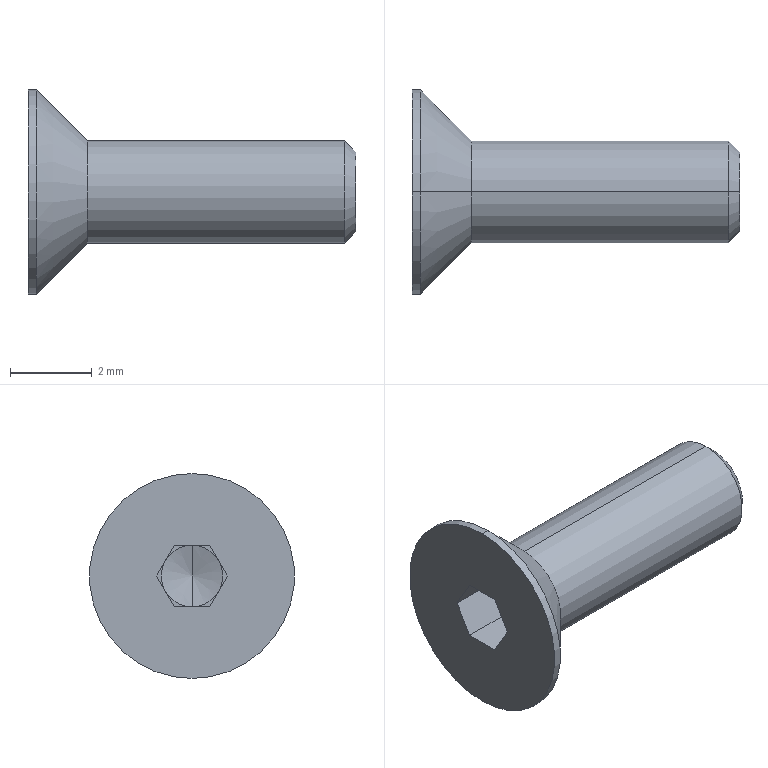Part | STEP file | 11-FG99-FBa2_5_8-V3.0-kkkkkk-998.11 | 1 solid | 24 faces | box 8 x 5 x 5 mm | volume 47.741 mm3 | plane 14 | cone 6 | cylinder 4 | commonest cylinder face diameters 2.5 x2 5 x2
STEP:
#1=CARTESIAN_POINT('',(1.361,0.,0.));
#2=VERTEX_POINT('',#1);
#3=CARTESIAN_POINT('',(1.16,0.,0.75));
#4=VERTEX_POINT('',#3);
#5=CARTESIAN_POINT('',(1.361,0.,0.));
#6=DIRECTION('',(-0.2588,0.,0.9659));
#7=VECTOR('',#6,1000.);
#8=LINE('',#5,#7);
#9=EDGE_CURVE('',#2,#4,#8,.T.);
#10=ORIENTED_EDGE('',*,*,#9,.F.);
#11=CARTESIAN_POINT('',(1.16,0.,-0.75));
#12=VERTEX_POINT('',#11);
#13=CARTESIAN_POINT('',(1.361,0.,0.));
#14=DIRECTION('',(-0.2588,0.,-0.9659));
#15=VECTOR('',#14,1000.);
#16=LINE('',#13,#15);
#17=EDGE_CURVE('',#2,#12,#16,.T.);
#18=ORIENTED_EDGE('',*,*,#17,.T.);
#19=CARTESIAN_POINT('',(1.16,-0.6495,-0.375));
#20=VERTEX_POINT('',#19);
#21=CARTESIAN_POINT('',(1.16,0.,0.));
#22=DIRECTION('',(-1.,0.,0.));
#23=DIRECTION('',(0.,0.,1.));
#24=AXIS2_PLACEMENT_3D('',#21,#22,#23);
#25=CIRCLE('',#24,0.75);
#26=EDGE_CURVE('',#12,#20,#25,.T.);
#27=ORIENTED_EDGE('',*,*,#26,.T.);
#28=CARTESIAN_POINT('',(1.16,-0.6495,0.375));
#29=VERTEX_POINT('',#28);
#30=CARTESIAN_POINT('',(1.16,0.,0.));
#31=DIRECTION('',(-1.,0.,0.));
#32=DIRECTION('',(0.,0.,1.));
#33=AXIS2_PLACEMENT_3D('',#30,#31,#32);
#34=CIRCLE('',#33,0.75);
#35=EDGE_CURVE('',#20,#29,#34,.T.);
#36=ORIENTED_EDGE('',*,*,#35,.T.);
#37=CARTESIAN_POINT('',(1.16,0.,0.));
#38=DIRECTION('',(-1.,0.,0.));
#39=DIRECTION('',(0.,0.,1.));
#40=AXIS2_PLACEMENT_3D('',#37,#38,#39);
#41=CIRCLE('',#40,0.75);
#42=EDGE_CURVE('',#29,#4,#41,.T.);
#43=ORIENTED_EDGE('',*,*,#42,.T.);
#44=EDGE_LOOP('',(#10,#18,#27,#36,#43));
#45=FACE_OUTER_BOUND('',#44,.T.);
#46=CARTESIAN_POINT('',(-998.639,0.,0.));
#47=DIRECTION('',(-1.,0.,0.));
#48=DIRECTION('',(0.,0.,1.));
#49=AXIS2_PLACEMENT_3D('',#46,#47,#48);
#50=CONICAL_SURFACE('',#49,3732.051,1.309);
#51=ADVANCED_FACE('',(#45),#50,.F.);
#52=CARTESIAN_POINT('',(8.,0.,0.974));
#53=VERTEX_POINT('',#52);
#54=CARTESIAN_POINT('',(8.,0.,-0.974));
#55=VERTEX_POINT('',#54);
#56=CARTESIAN_POINT('',(8.,0.,0.));
#57=DIRECTION('',(-1.,0.,0.));
#58=DIRECTION('',(0.,0.,1.));
#59=AXIS2_PLACEMENT_3D('',#56,#57,#58);
#60=CIRCLE('',#59,0.974);
#61=EDGE_CURVE('',#53,#55,#60,.T.);
#62=ORIENTED_EDGE('',*,*,#61,.T.);
#63=CARTESIAN_POINT('',(7.724,0.,-1.25));
#64=VERTEX_POINT('',#63);
#65=CARTESIAN_POINT('',(8.,0.,-0.974));
#66=DIRECTION('',(-0.7071,0.,-0.7071));
#67=VECTOR('',#66,1000.);
#68=LINE('',#65,#67);
#69=EDGE_CURVE('',#55,#64,#68,.T.);
#70=ORIENTED_EDGE('',*,*,#69,.T.);
#71=CARTESIAN_POINT('',(7.724,0.,1.25));
#72=VERTEX_POINT('',#71);
#73=CARTESIAN_POINT('',(7.724,0.,0.));
#74=DIRECTION('',(-1.,0.,0.));
#75=DIRECTION('',(0.,0.,1.));
#76=AXIS2_PLACEMENT_3D('',#73,#74,#75);
#77=CIRCLE('',#76,1.25);
#78=EDGE_CURVE('',#72,#64,#77,.T.);
#79=ORIENTED_EDGE('',*,*,#78,.F.);
#80=CARTESIAN_POINT('',(8.,0.,0.974));
#81=DIRECTION('',(-0.7071,0.,0.7071));
#82=VECTOR('',#81,1000.);
#83=LINE('',#80,#82);
#84=EDGE_CURVE('',#53,#72,#83,.T.);
#85=ORIENTED_EDGE('',*,*,#84,.F.);
#86=EDGE_LOOP('',(#62,#70,#79,#85));
#87=FACE_OUTER_BOUND('',#86,.T.);
#88=CARTESIAN_POINT('',(8.,0.,0.));
#89=DIRECTION('',(-1.,0.,0.));
#90=DIRECTION('',(0.,0.,1.));
#91=AXIS2_PLACEMENT_3D('',#88,#89,#90);
#92=CONICAL_SURFACE('',#91,0.974,0.7854);
#93=ADVANCED_FACE('',(#87),#92,.T.);
#94=ORIENTED_EDGE('',*,*,#78,.T.);
#95=CARTESIAN_POINT('',(1.45,0.,-1.25));
#96=VERTEX_POINT('',#95);
#97=CARTESIAN_POINT('',(8.,0.,-1.25));
#98=DIRECTION('',(-1.,0.,0.));
#99=VECTOR('',#98,1000.);
#100=LINE('',#97,#99);
#101=EDGE_CURVE('',#64,#96,#100,.T.);
#102=ORIENTED_EDGE('',*,*,#101,.T.);
#103=CARTESIAN_POINT('',(1.45,0.,1.25));
#104=VERTEX_POINT('',#103);
#105=CARTESIAN_POINT('',(1.45,0.,0.));
#106=DIRECTION('',(-1.,0.,0.));
#107=DIRECTION('',(0.,0.,1.));
#108=AXIS2_PLACEMENT_3D('',#105,#106,#107);
#109=CIRCLE('',#108,1.25);
#110=EDGE_CURVE('',#104,#96,#109,.T.);
#111=ORIENTED_EDGE('',*,*,#110,.F.);
#112=CARTESIAN_POINT('',(8.,0.,1.25));
#113=DIRECTION('',(-1.,0.,0.));
#114=VECTOR('',#113,1000.);
#115=LINE('',#112,#114);
#116=EDGE_CURVE('',#72,#104,#115,.T.);
#117=ORIENTED_EDGE('',*,*,#116,.F.);
#118=EDGE_LOOP('',(#94,#102,#111,#117));
#119=FACE_OUTER_BOUND('',#118,.T.);
#120=CARTESIAN_POINT('',(8.,0.,0.));
#121=DIRECTION('',(-1.,0.,0.));
#122=DIRECTION('',(0.,0.,1.));
#123=AXIS2_PLACEMENT_3D('',#120,#121,#122);
#124=CYLINDRICAL_SURFACE('',#123,1.25);
#125=ADVANCED_FACE('',(#119),#124,.T.);
#126=ORIENTED_EDGE('',*,*,#110,.T.);
#127=CARTESIAN_POINT('',(0.2,0.,-2.5));
#128=VERTEX_POINT('',#127);
#129=CARTESIAN_POINT('',(1.45,0.,-1.25));
#130=DIRECTION('',(-0.7071,0.,-0.7071));
#131=VECTOR('',#130,1000.);
#132=LINE('',#129,#131);
#133=EDGE_CURVE('',#96,#128,#132,.T.);
#134=ORIENTED_EDGE('',*,*,#133,.T.);
#135=CARTESIAN_POINT('',(0.2,0.,2.5));
#136=VERTEX_POINT('',#135);
#137=CARTESIAN_POINT('',(0.2,0.,0.));
#138=DIRECTION('',(-1.,0.,0.));
#139=DIRECTION('',(0.,0.,1.));
#140=AXIS2_PLACEMENT_3D('',#137,#138,#139);
#141=CIRCLE('',#140,2.5);
#142=EDGE_CURVE('',#136,#128,#141,.T.);
#143=ORIENTED_EDGE('',*,*,#142,.F.);
#144=CARTESIAN_POINT('',(1.45,0.,1.25));
#145=DIRECTION('',(-0.7071,0.,0.7071));
#146=VECTOR('',#145,1000.);
#147=LINE('',#144,#146);
#148=EDGE_CURVE('',#104,#136,#147,.T.);
#149=ORIENTED_EDGE('',*,*,#148,.F.);
#150=EDGE_LOOP('',(#126,#134,#143,#149));
#151=FACE_OUTER_BOUND('',#150,.T.);
#152=CARTESIAN_POINT('',(1.45,0.,0.));
#153=DIRECTION('',(-1.,0.,0.));
#154=DIRECTION('',(0.,0.,1.));
#155=AXIS2_PLACEMENT_3D('',#152,#153,#154);
#156=CONICAL_SURFACE('',#155,1.25,0.7854);
#157=ADVANCED_FACE('',(#151),#156,.T.);
#158=ORIENTED_EDGE('',*,*,#142,.T.);
#159=CARTESIAN_POINT('',(0.,0.,-2.5));
#160=VERTEX_POINT('',#159);
#161=CARTESIAN_POINT('',(8.,0.,-2.5));
#162=DIRECTION('',(-1.,0.,0.));
#163=VECTOR('',#162,1000.);
#164=LINE('',#161,#163);
#165=EDGE_CURVE('',#128,#160,#164,.T.);
#166=ORIENTED_EDGE('',*,*,#165,.T.);
#167=CARTESIAN_POINT('',(0.,0.,2.5));
#168=VERTEX_POINT('',#167);
#169=CARTESIAN_POINT('',(0.,0.,0.));
#170=DIRECTION('',(-1.,0.,0.));
#171=DIRECTION('',(0.,0.,1.));
#172=AXIS2_PLACEMENT_3D('',#169,#170,#171);
#173=CIRCLE('',#172,2.5);
#174=EDGE_CURVE('',#168,#160,#173,.T.);
#175=ORIENTED_EDGE('',*,*,#174,.F.);
#176=CARTESIAN_POINT('',(8.,0.,2.5));
#177=DIRECTION('',(-1.,0.,0.));
#178=VECTOR('',#177,1000.);
#179=LINE('',#176,#178);
#180=EDGE_CURVE('',#136,#168,#179,.T.);
#181=ORIENTED_EDGE('',*,*,#180,.F.);
#182=EDGE_LOOP('',(#158,#166,#175,#181));
#183=FACE_OUTER_BOUND('',#182,.T.);
#184=CARTESIAN_POINT('',(8.,0.,0.));
#185=DIRECTION('',(-1.,0.,0.));
#186=DIRECTION('',(0.,0.,1.));
#187=AXIS2_PLACEMENT_3D('',#184,#185,#186);
#188=CYLINDRICAL_SURFACE('',#187,2.5);
#189=ADVANCED_FACE('',(#183),#188,.T.);
#190=ORIENTED_EDGE('',*,*,#174,.T.);
#191=CARTESIAN_POINT('',(0.,0.,0.));
#192=DIRECTION('',(-1.,0.,0.));
#193=DIRECTION('',(0.,0.,1.));
#194=AXIS2_PLACEMENT_3D('',#191,#192,#193);
#195=CIRCLE('',#194,2.5);
#196=EDGE_CURVE('',#160,#168,#195,.T.);
#197=ORIENTED_EDGE('',*,*,#196,.T.);
#198=EDGE_LOOP('',(#190,#197));
#199=FACE_OUTER_BOUND('',#198,.T.);
#200=CARTESIAN_POINT('',(0.,-0.433,0.75));
#201=VERTEX_POINT('',#200);
#202=CARTESIAN_POINT('',(0.,-0.866,0.));
#203=VERTEX_POINT('',#202);
#204=CARTESIAN_POINT('',(0.,-0.433,0.75));
#205=DIRECTION('',(0.,-0.5,-0.866));
#206=VECTOR('',#205,1000.);
#207=LINE('',#204,#206);
#208=EDGE_CURVE('',#201,#203,#207,.T.);
#209=ORIENTED_EDGE('',*,*,#208,.T.);
#210=CARTESIAN_POINT('',(0.,-0.433,-0.75));
#211=VERTEX_POINT('',#210);
#212=CARTESIAN_POINT('',(0.,-0.866,0.));
#213=DIRECTION('',(0.,0.5,-0.866));
#214=VECTOR('',#213,1000.);
#215=LINE('',#212,#214);
#216=EDGE_CURVE('',#203,#211,#215,.T.);
#217=ORIENTED_EDGE('',*,*,#216,.T.);
#218=CARTESIAN_POINT('',(0.,0.433,-0.75));
#219=VERTEX_POINT('',#218);
#220=CARTESIAN_POINT('',(0.,-0.433,-0.75));
#221=DIRECTION('',(0.,1.,0.));
#222=VECTOR('',#221,1000.);
#223=LINE('',#220,#222);
#224=EDGE_CURVE('',#211,#219,#223,.T.);
#225=ORIENTED_EDGE('',*,*,#224,.T.);
#226=CARTESIAN_POINT('',(0.,0.866,0.));
#227=VERTEX_POINT('',#226);
#228=CARTESIAN_POINT('',(0.,0.433,-0.75));
#229=DIRECTION('',(0.,0.5,0.866));
#230=VECTOR('',#229,1000.);
#231=LINE('',#228,#230);
#232=EDGE_CURVE('',#219,#227,#231,.T.);
#233=ORIENTED_EDGE('',*,*,#232,.T.);
#234=CARTESIAN_POINT('',(0.,0.433,0.75));
#235=VERTEX_POINT('',#234);
#236=CARTESIAN_POINT('',(0.,0.866,0.));
#237=DIRECTION('',(0.,-0.5,0.866));
#238=VECTOR('',#237,1000.);
#239=LINE('',#236,#238);
#240=EDGE_CURVE('',#227,#235,#239,.T.);
#241=ORIENTED_EDGE('',*,*,#240,.T.);
#242=CARTESIAN_POINT('',(0.,0.433,0.75));
#243=DIRECTION('',(0.,-1.,0.));
#244=VECTOR('',#243,1000.);
#245=LINE('',#242,#244);
#246=EDGE_CURVE('',#235,#201,#245,.T.);
#247=ORIENTED_EDGE('',*,*,#246,.T.);
#248=EDGE_LOOP('',(#209,#217,#225,#233,#241,#247));
#249=FACE_BOUND('',#248,.T.);
#250=CARTESIAN_POINT('',(0.,0.,0.));
#251=DIRECTION('',(1.,0.,0.));
#252=DIRECTION('',(0.,0.,-1.));
#253=AXIS2_PLACEMENT_3D('',#250,#251,#252);
#254=PLANE('',#253);
#255=ADVANCED_FACE('',(#199,#249),#254,.F.);
#256=ORIENTED_EDGE('',*,*,#165,.F.);
#257=CARTESIAN_POINT('',(0.2,0.,0.));
#258=DIRECTION('',(-1.,0.,0.));
#259=DIRECTION('',(0.,0.,1.));
#260=AXIS2_PLACEMENT_3D('',#257,#258,#259);
#261=CIRCLE('',#260,2.5);
#262=EDGE_CURVE('',#128,#136,#261,.T.);
#263=ORIENTED_EDGE('',*,*,#262,.T.);
#264=ORIENTED_EDGE('',*,*,#180,.T.);
#265=ORIENTED_EDGE('',*,*,#196,.F.);
#266=EDGE_LOOP('',(#256,#263,#264,#265));
#267=FACE_OUTER_BOUND('',#266,.T.);
#268=CARTESIAN_POINT('',(8.,0.,0.));
#269=DIRECTION('',(-1.,0.,0.));
#270=DIRECTION('',(0.,0.,1.));
#271=AXIS2_PLACEMENT_3D('',#268,#269,#270);
#272=CYLINDRICAL_SURFACE('',#271,2.5);
#273=ADVANCED_FACE('',(#267),#272,.T.);
#274=ORIENTED_EDGE('',*,*,#133,.F.);
#275=CARTESIAN_POINT('',(1.45,0.,0.));
#276=DIRECTION('',(-1.,0.,0.));
#277=DIRECTION('',(0.,0.,1.));
#278=AXIS2_PLACEMENT_3D('',#275,#276,#277);
#279=CIRCLE('',#278,1.25);
#280=EDGE_CURVE('',#96,#104,#279,.T.);
#281=ORIENTED_EDGE('',*,*,#280,.T.);
#282=ORIENTED_EDGE('',*,*,#148,.T.);
#283=ORIENTED_EDGE('',*,*,#262,.F.);
#284=EDGE_LOOP('',(#274,#281,#282,#283));
#285=FACE_OUTER_BOUND('',#284,.T.);
#286=CARTESIAN_POINT('',(1.45,0.,0.));
#287=DIRECTION('',(-1.,0.,0.));
#288=DIRECTION('',(0.,0.,1.));
#289=AXIS2_PLACEMENT_3D('',#286,#287,#288);
#290=CONICAL_SURFACE('',#289,1.25,0.7854);
#291=ADVANCED_FACE('',(#285),#290,.T.);
#292=ORIENTED_EDGE('',*,*,#101,.F.);
#293=CARTESIAN_POINT('',(7.724,0.,0.));
#294=DIRECTION('',(-1.,0.,0.));
#295=DIRECTION('',(0.,0.,1.));
#296=AXIS2_PLACEMENT_3D('',#293,#294,#295);
#297=CIRCLE('',#296,1.25);
#298=EDGE_CURVE('',#64,#72,#297,.T.);
#299=ORIENTED_EDGE('',*,*,#298,.T.);
#300=ORIENTED_EDGE('',*,*,#116,.T.);
#301=ORIENTED_EDGE('',*,*,#280,.F.);
#302=EDGE_LOOP('',(#292,#299,#300,#301));
#303=FACE_OUTER_BOUND('',#302,.T.);
#304=CARTESIAN_POINT('',(8.,0.,0.));
#305=DIRECTION('',(-1.,0.,0.));
#306=DIRECTION('',(0.,0.,1.));
#307=AXIS2_PLACEMENT_3D('',#304,#305,#306);
#308=CYLINDRICAL_SURFACE('',#307,1.25);
#309=ADVANCED_FACE('',(#303),#308,.T.);
#310=ORIENTED_EDGE('',*,*,#69,.F.);
#311=CARTESIAN_POINT('',(8.,0.,0.));
#312=DIRECTION('',(-1.,0.,0.));
#313=DIRECTION('',(0.,0.,1.));
#314=AXIS2_PLACEMENT_3D('',#311,#312,#313);
#315=CIRCLE('',#314,0.974);
#316=EDGE_CURVE('',#55,#53,#315,.T.);
#317=ORIENTED_EDGE('',*,*,#316,.T.);
#318=ORIENTED_EDGE('',*,*,#84,.T.);
#319=ORIENTED_EDGE('',*,*,#298,.F.);
#320=EDGE_LOOP('',(#310,#317,#318,#319));
#321=FACE_OUTER_BOUND('',#320,.T.);
#322=CARTESIAN_POINT('',(8.,0.,0.));
#323=DIRECTION('',(-1.,0.,0.));
#324=DIRECTION('',(0.,0.,1.));
#325=AXIS2_PLACEMENT_3D('',#322,#323,#324);
#326=CONICAL_SURFACE('',#325,0.974,0.7854);
#327=ADVANCED_FACE('',(#321),#326,.T.);
#328=ORIENTED_EDGE('',*,*,#61,.F.);
#329=ORIENTED_EDGE('',*,*,#316,.F.);
#330=EDGE_LOOP('',(#328,#329));
#331=FACE_OUTER_BOUND('',#330,.T.);
#332=CARTESIAN_POINT('',(8.,0.974,0.));
#333=DIRECTION('',(-1.,0.,0.));
#334=DIRECTION('',(0.,0.,1.));
#335=AXIS2_PLACEMENT_3D('',#332,#333,#334);
#336=PLANE('',#335);
#337=ADVANCED_FACE('',(#331),#336,.F.);
#338=CARTESIAN_POINT('',(1.16,0.866,0.));
#339=VERTEX_POINT('',#338);
#340=CARTESIAN_POINT('',(1.16,0.6495,0.375));
#341=VERTEX_POINT('',#340);
#342=CARTESIAN_POINT('',(1.16,0.866,0.));
#343=DIRECTION('',(0.,-0.5,0.866));
#344=VECTOR('',#343,1000.);
#345=LINE('',#342,#344);
#346=EDGE_CURVE('',#339,#341,#345,.T.);
#347=ORIENTED_EDGE('',*,*,#346,.T.);
#348=CARTESIAN_POINT('',(1.16,0.433,0.75));
#349=VERTEX_POINT('',#348);
#350=CARTESIAN_POINT('',(1.16,0.866,0.));
#351=DIRECTION('',(0.,-0.5,0.866));
#352=VECTOR('',#351,1000.);
#353=LINE('',#350,#352);
#354=EDGE_CURVE('',#341,#349,#353,.T.);
#355=ORIENTED_EDGE('',*,*,#354,.T.);
#356=CARTESIAN_POINT('',(1.16,0.433,0.75));
#357=DIRECTION('',(-1.,0.,0.));
#358=VECTOR('',#357,1000.);
#359=LINE('',#356,#358);
#360=EDGE_CURVE('',#349,#235,#359,.T.);
#361=ORIENTED_EDGE('',*,*,#360,.T.);
#362=ORIENTED_EDGE('',*,*,#240,.F.);
#363=CARTESIAN_POINT('',(1.16,0.866,0.));
#364=DIRECTION('',(-1.,0.,0.));
#365=VECTOR('',#364,1000.);
#366=LINE('',#363,#365);
#367=EDGE_CURVE('',#339,#227,#366,.T.);
#368=ORIENTED_EDGE('',*,*,#367,.F.);
#369=EDGE_LOOP('',(#347,#355,#361,#362,#368));
#370=FACE_OUTER_BOUND('',#369,.T.);
#371=CARTESIAN_POINT('',(1.16,0.866,0.));
#372=DIRECTION('',(0.,-0.866,-0.5));
#373=DIRECTION('',(0.,0.5,-0.866));
#374=AXIS2_PLACEMENT_3D('',#371,#372,#373);
#375=PLANE('',#374);
#376=ADVANCED_FACE('',(#370),#375,.T.);
#377=CARTESIAN_POINT('',(1.16,0.433,0.75));
#378=DIRECTION('',(0.,-1.,0.));
#379=VECTOR('',#378,1000.);
#380=LINE('',#377,#379);
#381=EDGE_CURVE('',#349,#4,#380,.T.);
#382=ORIENTED_EDGE('',*,*,#381,.T.);
#383=CARTESIAN_POINT('',(1.16,-0.433,0.75));
#384=VERTEX_POINT('',#383);
#385=CARTESIAN_POINT('',(1.16,0.433,0.75));
#386=DIRECTION('',(0.,-1.,0.));
#387=VECTOR('',#386,1000.);
#388=LINE('',#385,#387);
#389=EDGE_CURVE('',#4,#384,#388,.T.);
#390=ORIENTED_EDGE('',*,*,#389,.T.);
#391=CARTESIAN_POINT('',(1.16,-0.433,0.75));
#392=DIRECTION('',(-1.,0.,0.));
#393=VECTOR('',#392,1000.);
#394=LINE('',#391,#393);
#395=EDGE_CURVE('',#384,#201,#394,.T.);
#396=ORIENTED_EDGE('',*,*,#395,.T.);
#397=ORIENTED_EDGE('',*,*,#246,.F.);
#398=ORIENTED_EDGE('',*,*,#360,.F.);
#399=EDGE_LOOP('',(#382,#390,#396,#397,#398));
#400=FACE_OUTER_BOUND('',#399,.T.);
#401=CARTESIAN_POINT('',(1.16,0.433,0.75));
#402=DIRECTION('',(0.,0.,-1.));
#403=DIRECTION('',(-1.,0.,0.));
#404=AXIS2_PLACEMENT_3D('',#401,#402,#403);
#405=PLANE('',#404);
#406=ADVANCED_FACE('',(#400),#405,.T.);
#407=CARTESIAN_POINT('',(1.16,-0.433,0.75));
#408=DIRECTION('',(0.,-0.5,-0.866));
#409=VECTOR('',#408,1000.);
#410=LINE('',#407,#409);
#411=EDGE_CURVE('',#384,#29,#410,.T.);
#412=ORIENTED_EDGE('',*,*,#411,.T.);
#413=CARTESIAN_POINT('',(1.16,-0.866,0.));
#414=VERTEX_POINT('',#413);
#415=CARTESIAN_POINT('',(1.16,-0.433,0.75));
#416=DIRECTION('',(0.,-0.5,-0.866));
#417=VECTOR('',#416,1000.);
#418=LINE('',#415,#417);
#419=EDGE_CURVE('',#29,#414,#418,.T.);
#420=ORIENTED_EDGE('',*,*,#419,.T.);
#421=CARTESIAN_POINT('',(1.16,-0.866,0.));
#422=DIRECTION('',(-1.,0.,0.));
#423=VECTOR('',#422,1000.);
#424=LINE('',#421,#423);
#425=EDGE_CURVE('',#414,#203,#424,.T.);
#426=ORIENTED_EDGE('',*,*,#425,.T.);
#427=ORIENTED_EDGE('',*,*,#208,.F.);
#428=ORIENTED_EDGE('',*,*,#395,.F.);
#429=EDGE_LOOP('',(#412,#420,#426,#427,#428));
#430=FACE_OUTER_BOUND('',#429,.T.);
#431=CARTESIAN_POINT('',(1.16,-0.433,0.75));
#432=DIRECTION('',(0.,0.866,-0.5));
#433=DIRECTION('',(0.,0.5,0.866));
#434=AXIS2_PLACEMENT_3D('',#431,#432,#433);
#435=PLANE('',#434);
#436=ADVANCED_FACE('',(#430),#435,.T.);
#437=CARTESIAN_POINT('',(1.16,-0.866,0.));
#438=DIRECTION('',(0.,0.5,-0.866));
#439=VECTOR('',#438,1000.);
#440=LINE('',#437,#439);
#441=EDGE_CURVE('',#414,#20,#440,.T.);
#442=ORIENTED_EDGE('',*,*,#441,.T.);
#443=CARTESIAN_POINT('',(1.16,-0.433,-0.75));
#444=VERTEX_POINT('',#443);
#445=CARTESIAN_POINT('',(1.16,-0.866,0.));
#446=DIRECTION('',(0.,0.5,-0.866));
#447=VECTOR('',#446,1000.);
#448=LINE('',#445,#447);
#449=EDGE_CURVE('',#20,#444,#448,.T.);
#450=ORIENTED_EDGE('',*,*,#449,.T.);
#451=CARTESIAN_POINT('',(1.16,-0.433,-0.75));
#452=DIRECTION('',(-1.,0.,0.));
#453=VECTOR('',#452,1000.);
#454=LINE('',#451,#453);
#455=EDGE_CURVE('',#444,#211,#454,.T.);
#456=ORIENTED_EDGE('',*,*,#455,.T.);
#457=ORIENTED_EDGE('',*,*,#216,.F.);
#458=ORIENTED_EDGE('',*,*,#425,.F.);
#459=EDGE_LOOP('',(#442,#450,#456,#457,#458));
#460=FACE_OUTER_BOUND('',#459,.T.);
#461=CARTESIAN_POINT('',(1.16,-0.866,0.));
#462=DIRECTION('',(0.,0.866,0.5));
#463=DIRECTION('',(0.,-0.5,0.866));
#464=AXIS2_PLACEMENT_3D('',#461,#462,#463);
#465=PLANE('',#464);
#466=ADVANCED_FACE('',(#460),#465,.T.);
#467=CARTESIAN_POINT('',(1.16,-0.433,-0.75));
#468=DIRECTION('',(0.,1.,0.));
#469=VECTOR('',#468,1000.);
#470=LINE('',#467,#469);
#471=EDGE_CURVE('',#444,#12,#470,.T.);
#472=ORIENTED_EDGE('',*,*,#471,.T.);
#473=CARTESIAN_POINT('',(1.16,0.433,-0.75));
#474=VERTEX_POINT('',#473);
#475=CARTESIAN_POINT('',(1.16,-0.433,-0.75));
#476=DIRECTION('',(0.,1.,0.));
#477=VECTOR('',#476,1000.);
#478=LINE('',#475,#477);
#479=EDGE_CURVE('',#12,#474,#478,.T.);
#480=ORIENTED_EDGE('',*,*,#479,.T.);
#481=CARTESIAN_POINT('',(1.16,0.433,-0.75));
#482=DIRECTION('',(-1.,0.,0.));
#483=VECTOR('',#482,1000.);
#484=LINE('',#481,#483);
#485=EDGE_CURVE('',#474,#219,#484,.T.);
#486=ORIENTED_EDGE('',*,*,#485,.T.);
#487=ORIENTED_EDGE('',*,*,#224,.F.);
#488=ORIENTED_EDGE('',*,*,#455,.F.);
#489=EDGE_LOOP('',(#472,#480,#486,#487,#488));
#490=FACE_OUTER_BOUND('',#489,.T.);
#491=CARTESIAN_POINT('',(1.16,-0.433,-0.75));
#492=DIRECTION('',(0.,0.,1.));
#493=DIRECTION('',(1.,0.,0.));
#494=AXIS2_PLACEMENT_3D('',#491,#492,#493);
#495=PLANE('',#494);
#496=ADVANCED_FACE('',(#490),#495,.T.);
#497=CARTESIAN_POINT('',(1.16,0.6495,-0.375));
#498=VERTEX_POINT('',#497);
#499=CARTESIAN_POINT('',(1.16,0.433,-0.75));
#500=DIRECTION('',(0.,0.5,0.866));
#501=VECTOR('',#500,1000.);
#502=LINE('',#499,#501);
#503=EDGE_CURVE('',#474,#498,#502,.T.);
#504=ORIENTED_EDGE('',*,*,#503,.T.);
#505=CARTESIAN_POINT('',(1.16,0.433,-0.75));
#506=DIRECTION('',(0.,0.5,0.866));
#507=VECTOR('',#506,1000.);
#508=LINE('',#505,#507);
#509=EDGE_CURVE('',#498,#339,#508,.T.);
#510=ORIENTED_EDGE('',*,*,#509,.T.);
#511=ORIENTED_EDGE('',*,*,#367,.T.);
#512=ORIENTED_EDGE('',*,*,#232,.F.);
#513=ORIENTED_EDGE('',*,*,#485,.F.);
#514=EDGE_LOOP('',(#504,#510,#511,#512,#513));
#515=FACE_OUTER_BOUND('',#514,.T.);
#516=CARTESIAN_POINT('',(1.16,0.433,-0.75));
#517=DIRECTION('',(0.,-0.866,0.5));
#518=DIRECTION('',(0.,-0.5,-0.866));
#519=AXIS2_PLACEMENT_3D('',#516,#517,#518);
#520=PLANE('',#519);
#521=ADVANCED_FACE('',(#515),#520,.T.);
#522=CARTESIAN_POINT('',(1.16,0.,0.));
#523=DIRECTION('',(-1.,0.,0.));
#524=DIRECTION('',(0.,0.,1.));
#525=AXIS2_PLACEMENT_3D('',#522,#523,#524);
#526=CIRCLE('',#525,0.75);
#527=EDGE_CURVE('',#498,#12,#526,.T.);
#528=ORIENTED_EDGE('',*,*,#527,.F.);
#529=ORIENTED_EDGE('',*,*,#503,.F.);
#530=ORIENTED_EDGE('',*,*,#479,.F.);
#531=EDGE_LOOP('',(#528,#529,#530));
#532=FACE_OUTER_BOUND('',#531,.T.);
#533=CARTESIAN_POINT('',(1.16,0.,0.));
#534=DIRECTION('',(1.,0.,0.));
#535=DIRECTION('',(0.,0.,-1.));
#536=AXIS2_PLACEMENT_3D('',#533,#534,#535);
#537=PLANE('',#536);
#538=ADVANCED_FACE('',(#532),#537,.F.);
#539=CARTESIAN_POINT('',(1.16,0.,0.));
#540=DIRECTION('',(-1.,0.,0.));
#541=DIRECTION('',(0.,0.,1.));
#542=AXIS2_PLACEMENT_3D('',#539,#540,#541);
#543=CIRCLE('',#542,0.75);
#544=EDGE_CURVE('',#341,#498,#543,.T.);
#545=ORIENTED_EDGE('',*,*,#544,.F.);
#546=ORIENTED_EDGE('',*,*,#346,.F.);
#547=ORIENTED_EDGE('',*,*,#509,.F.);
#548=EDGE_LOOP('',(#545,#546,#547));
#549=FACE_OUTER_BOUND('',#548,.T.);
#550=CARTESIAN_POINT('',(1.16,0.,0.));
#551=DIRECTION('',(1.,0.,0.));
#552=DIRECTION('',(0.,0.,-1.));
#553=AXIS2_PLACEMENT_3D('',#550,#551,#552);
#554=PLANE('',#553);
#555=ADVANCED_FACE('',(#549),#554,.F.);
#556=CARTESIAN_POINT('',(1.16,0.,0.));
#557=DIRECTION('',(-1.,0.,0.));
#558=DIRECTION('',(0.,0.,1.));
#559=AXIS2_PLACEMENT_3D('',#556,#557,#558);
#560=CIRCLE('',#559,0.75);
#561=EDGE_CURVE('',#4,#341,#560,.T.);
#562=ORIENTED_EDGE('',*,*,#561,.F.);
#563=ORIENTED_EDGE('',*,*,#381,.F.);
#564=ORIENTED_EDGE('',*,*,#354,.F.);
#565=EDGE_LOOP('',(#562,#563,#564));
#566=FACE_OUTER_BOUND('',#565,.T.);
#567=CARTESIAN_POINT('',(1.16,0.,0.));
#568=DIRECTION('',(1.,0.,0.));
#569=DIRECTION('',(0.,0.,-1.));
#570=AXIS2_PLACEMENT_3D('',#567,#568,#569);
#571=PLANE('',#570);
#572=ADVANCED_FACE('',(#566),#571,.F.);
#573=ORIENTED_EDGE('',*,*,#42,.F.);
#574=ORIENTED_EDGE('',*,*,#411,.F.);
#575=ORIENTED_EDGE('',*,*,#389,.F.);
#576=EDGE_LOOP('',(#573,#574,#575));
#577=FACE_OUTER_BOUND('',#576,.T.);
#578=CARTESIAN_POINT('',(1.16,0.,0.));
#579=DIRECTION('',(1.,0.,0.));
#580=DIRECTION('',(0.,0.,-1.));
#581=AXIS2_PLACEMENT_3D('',#578,#579,#580);
#582=PLANE('',#581);
#583=ADVANCED_FACE('',(#577),#582,.F.);
#584=ORIENTED_EDGE('',*,*,#35,.F.);
#585=ORIENTED_EDGE('',*,*,#441,.F.);
#586=ORIENTED_EDGE('',*,*,#419,.F.);
#587=EDGE_LOOP('',(#584,#585,#586));
#588=FACE_OUTER_BOUND('',#587,.T.);
#589=CARTESIAN_POINT('',(1.16,0.,0.));
#590=DIRECTION('',(1.,0.,0.));
#591=DIRECTION('',(0.,0.,-1.));
#592=AXIS2_PLACEMENT_3D('',#589,#590,#591);
#593=PLANE('',#592);
#594=ADVANCED_FACE('',(#588),#593,.F.);
#595=ORIENTED_EDGE('',*,*,#26,.F.);
#596=ORIENTED_EDGE('',*,*,#471,.F.);
#597=ORIENTED_EDGE('',*,*,#449,.F.);
#598=EDGE_LOOP('',(#595,#596,#597));
#599=FACE_OUTER_BOUND('',#598,.T.);
#600=CARTESIAN_POINT('',(1.16,0.,0.));
#601=DIRECTION('',(1.,0.,0.));
#602=DIRECTION('',(0.,0.,-1.));
#603=AXIS2_PLACEMENT_3D('',#600,#601,#602);
#604=PLANE('',#603);
#605=ADVANCED_FACE('',(#599),#604,.F.);
#606=ORIENTED_EDGE('',*,*,#17,.F.);
#607=ORIENTED_EDGE('',*,*,#9,.T.);
#608=ORIENTED_EDGE('',*,*,#561,.T.);
#609=ORIENTED_EDGE('',*,*,#544,.T.);
#610=ORIENTED_EDGE('',*,*,#527,.T.);
#611=EDGE_LOOP('',(#606,#607,#608,#609,#610));
#612=FACE_OUTER_BOUND('',#611,.T.);
#613=CARTESIAN_POINT('',(-998.639,0.,0.));
#614=DIRECTION('',(-1.,0.,0.));
#615=DIRECTION('',(0.,0.,1.));
#616=AXIS2_PLACEMENT_3D('',#613,#614,#615);
#617=CONICAL_SURFACE('',#616,3732.051,1.309);
#618=ADVANCED_FACE('',(#612),#617,.F.);
#619=CLOSED_SHELL('',(#51,#93,#125,#157,#189,#255,#273,#291,#309,#327,#337,#376,#406,#436,#466,#496,#521,#538,#555,#572,#583,#594,#605,#618));
#620=MANIFOLD_SOLID_BREP('',#619);
#621=CARTESIAN_POINT('',(0.,0.,0.));
#622=DIRECTION('',(0.,0.,1.));
#623=DIRECTION('',(1.,0.,0.));
#624=AXIS2_PLACEMENT_3D('',#621,#622,#623);
#625=(LENGTH_UNIT()NAMED_UNIT(*)SI_UNIT(.MILLI.,.METRE.));
#626=UNCERTAINTY_MEASURE_WITH_UNIT(LENGTH_MEASURE(0.00001),#625,'','');
#627=(NAMED_UNIT(*)PLANE_ANGLE_UNIT()SI_UNIT($,.RADIAN.));
#628=(NAMED_UNIT(*)SI_UNIT($,.STERADIAN.)SOLID_ANGLE_UNIT());
#629=(GEOMETRIC_REPRESENTATION_CONTEXT(3)GLOBAL_UNCERTAINTY_ASSIGNED_CONTEXT((#626))GLOBAL_UNIT_ASSIGNED_CONTEXT((#625,#627,#628))REPRESENTATION_CONTEXT('',''));
#630=ADVANCED_BREP_SHAPE_REPRESENTATION('',(#620,#624),#629);